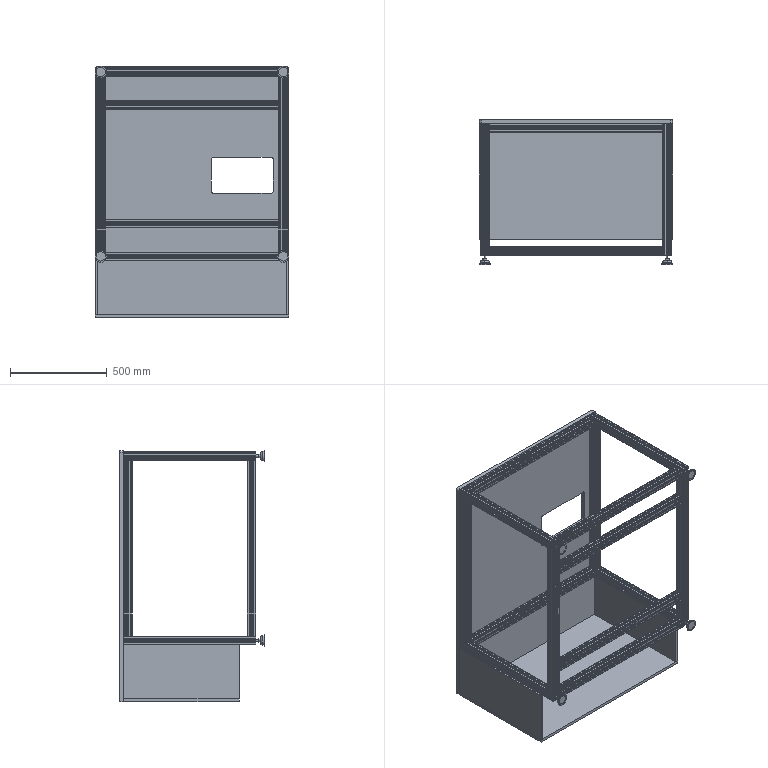Part | STEP file | Final inspection modification | 22 solids | 1820 faces | box 1005 x 750 x 1303 mm | volume 47486474 mm3 | plane 1220 | cylinder 576 | cone 16 | torus 8 | commonest cylinder face diameters 2 x252 3 x168 12.5 x70 6 x56 12 x8 48 x8